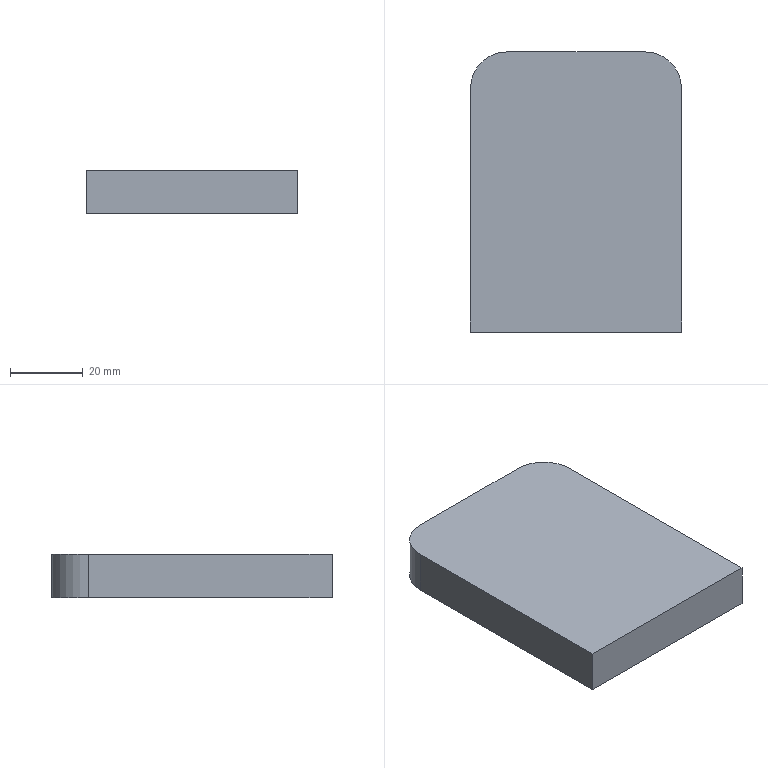Part | SolidWorks | features Extrusion 1, Fillet 1 | 1 solid | 8 faces | box 58 x 77 x 12 mm | volume 53077 mm3 | plane 6 | cylinder 2 | commonest cylinder face diameters 20 x2
STEP:
#1=CARTESIAN_POINT('',(29.,-38.5,0.));
#2=VERTEX_POINT('',#1);
#3=CARTESIAN_POINT('',(29.,28.5,0.));
#4=VERTEX_POINT('',#3);
#5=CARTESIAN_POINT('',(29.,-38.5,0.));
#6=DIRECTION('',(0.,1.,0.));
#7=VECTOR('',#6,1000.);
#8=LINE('',#5,#7);
#9=EDGE_CURVE('',#2,#4,#8,.T.);
#10=ORIENTED_EDGE('',*,*,#9,.T.);
#11=CARTESIAN_POINT('',(29.,28.5,12.));
#12=VERTEX_POINT('',#11);
#13=CARTESIAN_POINT('',(29.,28.5,12.));
#14=DIRECTION('',(0.,0.,1.));
#15=VECTOR('',#14,1000.);
#16=LINE('',#13,#15);
#17=EDGE_CURVE('',#4,#12,#16,.T.);
#18=ORIENTED_EDGE('',*,*,#17,.T.);
#19=CARTESIAN_POINT('',(29.,-38.5,12.));
#20=VERTEX_POINT('',#19);
#21=CARTESIAN_POINT('',(29.,-38.5,12.));
#22=DIRECTION('',(0.,1.,0.));
#23=VECTOR('',#22,1000.);
#24=LINE('',#21,#23);
#25=EDGE_CURVE('',#20,#12,#24,.T.);
#26=ORIENTED_EDGE('',*,*,#25,.F.);
#27=CARTESIAN_POINT('',(29.,-38.5,12.));
#28=DIRECTION('',(0.,0.,-1.));
#29=VECTOR('',#28,1000.);
#30=LINE('',#27,#29);
#31=EDGE_CURVE('',#20,#2,#30,.T.);
#32=ORIENTED_EDGE('',*,*,#31,.T.);
#33=EDGE_LOOP('',(#10,#18,#26,#32));
#34=FACE_OUTER_BOUND('',#33,.T.);
#35=CARTESIAN_POINT('',(29.,-38.5,12.));
#36=DIRECTION('',(-1.,0.,0.));
#37=DIRECTION('',(0.,0.,1.));
#38=AXIS2_PLACEMENT_3D('',#35,#36,#37);
#39=PLANE('',#38);
#40=ADVANCED_FACE('',(#34),#39,.F.);
#41=CARTESIAN_POINT('',(19.,38.5,0.));
#42=VERTEX_POINT('',#41);
#43=CARTESIAN_POINT('',(-19.,38.5,0.));
#44=VERTEX_POINT('',#43);
#45=CARTESIAN_POINT('',(-29.,38.5,0.));
#46=DIRECTION('',(-1.,0.,0.));
#47=VECTOR('',#46,1000.);
#48=LINE('',#45,#47);
#49=EDGE_CURVE('',#42,#44,#48,.T.);
#50=ORIENTED_EDGE('',*,*,#49,.T.);
#51=CARTESIAN_POINT('',(-19.,38.5,12.));
#52=VERTEX_POINT('',#51);
#53=CARTESIAN_POINT('',(-19.,38.5,12.));
#54=DIRECTION('',(0.,0.,1.));
#55=VECTOR('',#54,1000.);
#56=LINE('',#53,#55);
#57=EDGE_CURVE('',#44,#52,#56,.T.);
#58=ORIENTED_EDGE('',*,*,#57,.T.);
#59=CARTESIAN_POINT('',(19.,38.5,12.));
#60=VERTEX_POINT('',#59);
#61=CARTESIAN_POINT('',(-29.,38.5,12.));
#62=DIRECTION('',(-1.,0.,0.));
#63=VECTOR('',#62,1000.);
#64=LINE('',#61,#63);
#65=EDGE_CURVE('',#60,#52,#64,.T.);
#66=ORIENTED_EDGE('',*,*,#65,.F.);
#67=CARTESIAN_POINT('',(19.,38.5,12.));
#68=DIRECTION('',(0.,0.,-1.));
#69=VECTOR('',#68,1000.);
#70=LINE('',#67,#69);
#71=EDGE_CURVE('',#60,#42,#70,.T.);
#72=ORIENTED_EDGE('',*,*,#71,.T.);
#73=EDGE_LOOP('',(#50,#58,#66,#72));
#74=FACE_OUTER_BOUND('',#73,.T.);
#75=CARTESIAN_POINT('',(-29.,38.5,12.));
#76=DIRECTION('',(0.,-1.,0.));
#77=DIRECTION('',(0.,0.,-1.));
#78=AXIS2_PLACEMENT_3D('',#75,#76,#77);
#79=PLANE('',#78);
#80=ADVANCED_FACE('',(#74),#79,.F.);
#81=CARTESIAN_POINT('',(-29.,28.5,12.));
#82=VERTEX_POINT('',#81);
#83=CARTESIAN_POINT('',(-29.,-38.5,12.));
#84=VERTEX_POINT('',#83);
#85=CARTESIAN_POINT('',(-29.,-38.5,12.));
#86=DIRECTION('',(0.,-1.,0.));
#87=VECTOR('',#86,1000.);
#88=LINE('',#85,#87);
#89=EDGE_CURVE('',#82,#84,#88,.T.);
#90=ORIENTED_EDGE('',*,*,#89,.F.);
#91=CARTESIAN_POINT('',(-29.,28.5,0.));
#92=VERTEX_POINT('',#91);
#93=CARTESIAN_POINT('',(-29.,28.5,12.));
#94=DIRECTION('',(0.,0.,-1.));
#95=VECTOR('',#94,1000.);
#96=LINE('',#93,#95);
#97=EDGE_CURVE('',#82,#92,#96,.T.);
#98=ORIENTED_EDGE('',*,*,#97,.T.);
#99=CARTESIAN_POINT('',(-29.,-38.5,0.));
#100=VERTEX_POINT('',#99);
#101=CARTESIAN_POINT('',(-29.,-38.5,0.));
#102=DIRECTION('',(0.,-1.,0.));
#103=VECTOR('',#102,1000.);
#104=LINE('',#101,#103);
#105=EDGE_CURVE('',#92,#100,#104,.T.);
#106=ORIENTED_EDGE('',*,*,#105,.T.);
#107=CARTESIAN_POINT('',(-29.,-38.5,12.));
#108=DIRECTION('',(0.,0.,-1.));
#109=VECTOR('',#108,1000.);
#110=LINE('',#107,#109);
#111=EDGE_CURVE('',#84,#100,#110,.T.);
#112=ORIENTED_EDGE('',*,*,#111,.F.);
#113=EDGE_LOOP('',(#90,#98,#106,#112));
#114=FACE_OUTER_BOUND('',#113,.T.);
#115=CARTESIAN_POINT('',(-29.,-38.5,12.));
#116=DIRECTION('',(1.,0.,0.));
#117=DIRECTION('',(0.,0.,-1.));
#118=AXIS2_PLACEMENT_3D('',#115,#116,#117);
#119=PLANE('',#118);
#120=ADVANCED_FACE('',(#114),#119,.F.);
#121=CARTESIAN_POINT('',(-29.,-38.5,0.));
#122=DIRECTION('',(1.,0.,0.));
#123=VECTOR('',#122,1000.);
#124=LINE('',#121,#123);
#125=EDGE_CURVE('',#100,#2,#124,.T.);
#126=ORIENTED_EDGE('',*,*,#125,.T.);
#127=ORIENTED_EDGE('',*,*,#31,.F.);
#128=CARTESIAN_POINT('',(-29.,-38.5,12.));
#129=DIRECTION('',(1.,0.,0.));
#130=VECTOR('',#129,1000.);
#131=LINE('',#128,#130);
#132=EDGE_CURVE('',#84,#20,#131,.T.);
#133=ORIENTED_EDGE('',*,*,#132,.F.);
#134=ORIENTED_EDGE('',*,*,#111,.T.);
#135=EDGE_LOOP('',(#126,#127,#133,#134));
#136=FACE_OUTER_BOUND('',#135,.T.);
#137=CARTESIAN_POINT('',(-29.,-38.5,12.));
#138=DIRECTION('',(0.,1.,0.));
#139=DIRECTION('',(0.,0.,1.));
#140=AXIS2_PLACEMENT_3D('',#137,#138,#139);
#141=PLANE('',#140);
#142=ADVANCED_FACE('',(#136),#141,.F.);
#143=ORIENTED_EDGE('',*,*,#65,.T.);
#144=CARTESIAN_POINT('',(-19.,28.5,12.));
#145=DIRECTION('',(0.,0.,1.));
#146=DIRECTION('',(-1.,0.,0.));
#147=AXIS2_PLACEMENT_3D('',#144,#145,#146);
#148=CIRCLE('',#147,10.);
#149=EDGE_CURVE('',#52,#82,#148,.T.);
#150=ORIENTED_EDGE('',*,*,#149,.T.);
#151=ORIENTED_EDGE('',*,*,#89,.T.);
#152=ORIENTED_EDGE('',*,*,#132,.T.);
#153=ORIENTED_EDGE('',*,*,#25,.T.);
#154=CARTESIAN_POINT('',(19.,28.5,12.));
#155=DIRECTION('',(0.,0.,1.));
#156=DIRECTION('',(-1.,0.,0.));
#157=AXIS2_PLACEMENT_3D('',#154,#155,#156);
#158=CIRCLE('',#157,10.);
#159=EDGE_CURVE('',#12,#60,#158,.T.);
#160=ORIENTED_EDGE('',*,*,#159,.T.);
#161=EDGE_LOOP('',(#143,#150,#151,#152,#153,#160));
#162=FACE_OUTER_BOUND('',#161,.T.);
#163=CARTESIAN_POINT('',(0.,0.,12.));
#164=DIRECTION('',(0.,0.,-1.));
#165=DIRECTION('',(-1.,0.,0.));
#166=AXIS2_PLACEMENT_3D('',#163,#164,#165);
#167=PLANE('',#166);
#168=ADVANCED_FACE('',(#162),#167,.F.);
#169=ORIENTED_EDGE('',*,*,#105,.F.);
#170=CARTESIAN_POINT('',(-19.,28.5,0.));
#171=DIRECTION('',(0.,0.,-1.));
#172=DIRECTION('',(-1.,0.,0.));
#173=AXIS2_PLACEMENT_3D('',#170,#171,#172);
#174=CIRCLE('',#173,10.);
#175=EDGE_CURVE('',#92,#44,#174,.T.);
#176=ORIENTED_EDGE('',*,*,#175,.T.);
#177=ORIENTED_EDGE('',*,*,#49,.F.);
#178=CARTESIAN_POINT('',(19.,28.5,0.));
#179=DIRECTION('',(0.,0.,-1.));
#180=DIRECTION('',(-1.,0.,0.));
#181=AXIS2_PLACEMENT_3D('',#178,#179,#180);
#182=CIRCLE('',#181,10.);
#183=EDGE_CURVE('',#42,#4,#182,.T.);
#184=ORIENTED_EDGE('',*,*,#183,.T.);
#185=ORIENTED_EDGE('',*,*,#9,.F.);
#186=ORIENTED_EDGE('',*,*,#125,.F.);
#187=EDGE_LOOP('',(#169,#176,#177,#184,#185,#186));
#188=FACE_OUTER_BOUND('',#187,.T.);
#189=CARTESIAN_POINT('',(0.,0.,0.));
#190=DIRECTION('',(0.,0.,-1.));
#191=DIRECTION('',(-1.,0.,0.));
#192=AXIS2_PLACEMENT_3D('',#189,#190,#191);
#193=PLANE('',#192);
#194=ADVANCED_FACE('',(#188),#193,.T.);
#195=ORIENTED_EDGE('',*,*,#149,.F.);
#196=ORIENTED_EDGE('',*,*,#57,.F.);
#197=ORIENTED_EDGE('',*,*,#175,.F.);
#198=ORIENTED_EDGE('',*,*,#97,.F.);
#199=EDGE_LOOP('',(#195,#196,#197,#198));
#200=FACE_OUTER_BOUND('',#199,.T.);
#201=CARTESIAN_POINT('',(-19.,28.5,12.));
#202=DIRECTION('',(0.,0.,-1.));
#203=DIRECTION('',(-1.,0.,0.));
#204=AXIS2_PLACEMENT_3D('',#201,#202,#203);
#205=CYLINDRICAL_SURFACE('',#204,10.);
#206=ADVANCED_FACE('',(#200),#205,.T.);
#207=ORIENTED_EDGE('',*,*,#159,.F.);
#208=ORIENTED_EDGE('',*,*,#17,.F.);
#209=ORIENTED_EDGE('',*,*,#183,.F.);
#210=ORIENTED_EDGE('',*,*,#71,.F.);
#211=EDGE_LOOP('',(#207,#208,#209,#210));
#212=FACE_OUTER_BOUND('',#211,.T.);
#213=CARTESIAN_POINT('',(19.,28.5,12.));
#214=DIRECTION('',(0.,0.,-1.));
#215=DIRECTION('',(-1.,0.,0.));
#216=AXIS2_PLACEMENT_3D('',#213,#214,#215);
#217=CYLINDRICAL_SURFACE('',#216,10.);
#218=ADVANCED_FACE('',(#212),#217,.T.);
#219=CLOSED_SHELL('',(#40,#80,#120,#142,#168,#194,#206,#218));
#220=MANIFOLD_SOLID_BREP('',#219);
#221=CARTESIAN_POINT('',(0.,0.,0.));
#222=DIRECTION('',(0.,0.,1.));
#223=DIRECTION('',(1.,0.,0.));
#224=AXIS2_PLACEMENT_3D('',#221,#222,#223);
#225=(LENGTH_UNIT()NAMED_UNIT(*)SI_UNIT(.MILLI.,.METRE.));
#226=UNCERTAINTY_MEASURE_WITH_UNIT(LENGTH_MEASURE(0.00001),#225,'','');
#227=(NAMED_UNIT(*)PLANE_ANGLE_UNIT()SI_UNIT($,.RADIAN.));
#228=(NAMED_UNIT(*)SI_UNIT($,.STERADIAN.)SOLID_ANGLE_UNIT());
#229=(GEOMETRIC_REPRESENTATION_CONTEXT(3)GLOBAL_UNCERTAINTY_ASSIGNED_CONTEXT((#226))GLOBAL_UNIT_ASSIGNED_CONTEXT((#225,#227,#228))REPRESENTATION_CONTEXT('',''));
#230=ADVANCED_BREP_SHAPE_REPRESENTATION('',(#220,#224),#229);